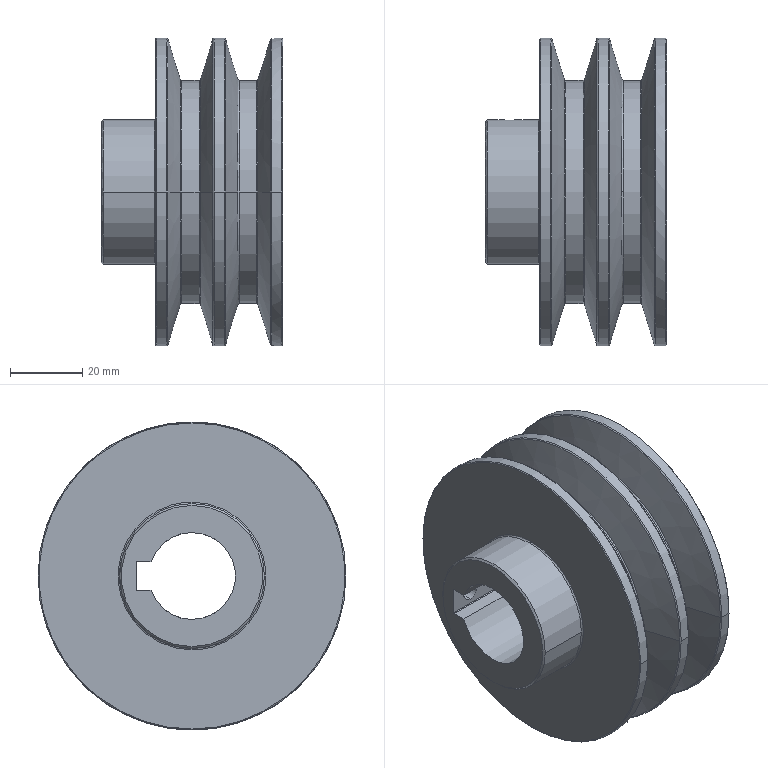Part | SolidWorks | features BaseBody 1 | 1 solid | 58 faces | box 50 x 85 x 85 mm | volume 143895 mm3 | cone 25 | cylinder 17 | spline 10 | plane 6 | commonest cylinder face diameters 85 x6 61.6 x4 0.32 x2 4.917 x2 40 x2 24 x1